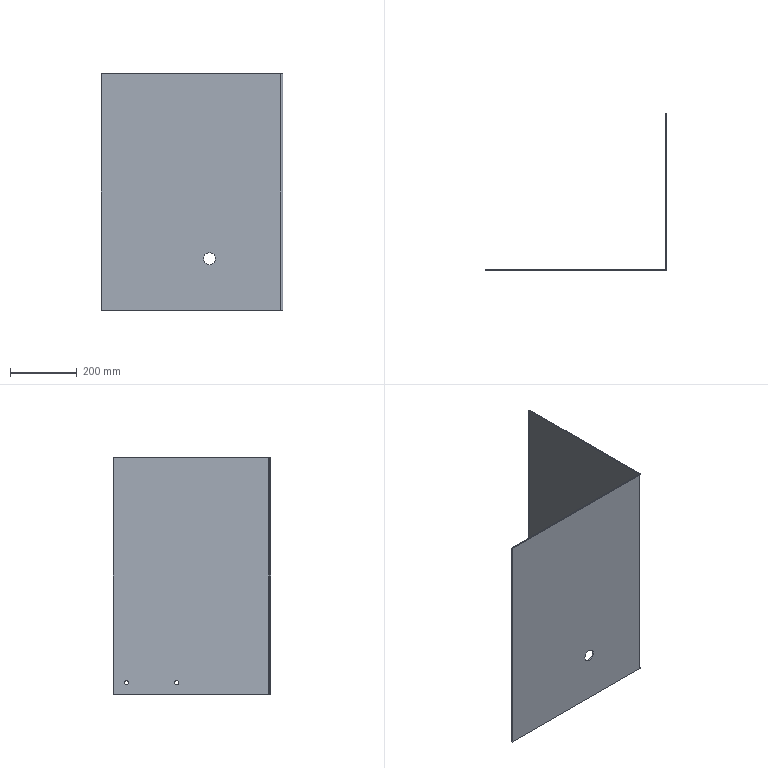Part | SolidWorks | features ICE 2, FlatPattern 1, SMBaseFlange 1, SheetMetal 1 | 1 solid | 20 faces | box 545 x 472 x 710 mm | volume 2151858 mm3 | plane 12 | cylinder 8 | commonest cylinder face diameters 12.7 x4 36.2 x2 6 x1 12 x1
STEP:
#1=CARTESIAN_POINT('',(-3.,432.,41.35));
#2=VERTEX_POINT('',#1);
#3=CARTESIAN_POINT('',(-3.,432.,28.65));
#4=VERTEX_POINT('',#3);
#5=CARTESIAN_POINT('',(-3.,432.,35.));
#6=DIRECTION('',(1.,0.,0.));
#7=DIRECTION('',(0.,0.,-1.));
#8=AXIS2_PLACEMENT_3D('',#5,#6,#7);
#9=CIRCLE('',#8,6.35);
#10=EDGE_CURVE('',#2,#4,#9,.T.);
#11=ORIENTED_EDGE('',*,*,#10,.F.);
#12=CARTESIAN_POINT('',(0.,432.,41.35));
#13=VERTEX_POINT('',#12);
#14=CARTESIAN_POINT('',(-10.,432.,41.35));
#15=DIRECTION('',(1.,0.,0.));
#16=VECTOR('',#15,1000.);
#17=LINE('',#14,#16);
#18=EDGE_CURVE('',#2,#13,#17,.T.);
#19=ORIENTED_EDGE('',*,*,#18,.T.);
#20=CARTESIAN_POINT('',(0.,432.,28.65));
#21=VERTEX_POINT('',#20);
#22=CARTESIAN_POINT('',(0.,432.,35.));
#23=DIRECTION('',(1.,0.,0.));
#24=DIRECTION('',(0.,0.,1.));
#25=AXIS2_PLACEMENT_3D('',#22,#23,#24);
#26=CIRCLE('',#25,6.35);
#27=EDGE_CURVE('',#13,#21,#26,.T.);
#28=ORIENTED_EDGE('',*,*,#27,.T.);
#29=CARTESIAN_POINT('',(-10.,432.,28.65));
#30=DIRECTION('',(1.,0.,0.));
#31=VECTOR('',#30,1000.);
#32=LINE('',#29,#31);
#33=EDGE_CURVE('',#4,#21,#32,.T.);
#34=ORIENTED_EDGE('',*,*,#33,.F.);
#35=EDGE_LOOP('',(#11,#19,#28,#34));
#36=FACE_OUTER_BOUND('',#35,.T.);
#37=CARTESIAN_POINT('',(-10.,432.,35.));
#38=DIRECTION('',(1.,0.,0.));
#39=DIRECTION('',(0.,0.,-1.));
#40=AXIS2_PLACEMENT_3D('',#37,#38,#39);
#41=CYLINDRICAL_SURFACE('',#40,6.35);
#42=ADVANCED_FACE('',(#36),#41,.F.);
#43=CARTESIAN_POINT('',(-3.,282.,41.35));
#44=VERTEX_POINT('',#43);
#45=CARTESIAN_POINT('',(-3.,282.,28.65));
#46=VERTEX_POINT('',#45);
#47=CARTESIAN_POINT('',(-3.,282.,35.));
#48=DIRECTION('',(1.,0.,0.));
#49=DIRECTION('',(0.,0.,-1.));
#50=AXIS2_PLACEMENT_3D('',#47,#48,#49);
#51=CIRCLE('',#50,6.35);
#52=EDGE_CURVE('',#44,#46,#51,.T.);
#53=ORIENTED_EDGE('',*,*,#52,.F.);
#54=CARTESIAN_POINT('',(0.,282.,41.35));
#55=VERTEX_POINT('',#54);
#56=CARTESIAN_POINT('',(-10.,282.,41.35));
#57=DIRECTION('',(1.,0.,0.));
#58=VECTOR('',#57,1000.);
#59=LINE('',#56,#58);
#60=EDGE_CURVE('',#44,#55,#59,.T.);
#61=ORIENTED_EDGE('',*,*,#60,.T.);
#62=CARTESIAN_POINT('',(0.,282.,28.65));
#63=VERTEX_POINT('',#62);
#64=CARTESIAN_POINT('',(0.,282.,35.));
#65=DIRECTION('',(1.,0.,0.));
#66=DIRECTION('',(0.,0.,1.));
#67=AXIS2_PLACEMENT_3D('',#64,#65,#66);
#68=CIRCLE('',#67,6.35);
#69=EDGE_CURVE('',#55,#63,#68,.T.);
#70=ORIENTED_EDGE('',*,*,#69,.T.);
#71=CARTESIAN_POINT('',(-10.,282.,28.65));
#72=DIRECTION('',(1.,0.,0.));
#73=VECTOR('',#72,1000.);
#74=LINE('',#71,#73);
#75=EDGE_CURVE('',#46,#63,#74,.T.);
#76=ORIENTED_EDGE('',*,*,#75,.F.);
#77=EDGE_LOOP('',(#53,#61,#70,#76));
#78=FACE_OUTER_BOUND('',#77,.T.);
#79=CARTESIAN_POINT('',(-10.,282.,35.));
#80=DIRECTION('',(1.,0.,0.));
#81=DIRECTION('',(0.,0.,-1.));
#82=AXIS2_PLACEMENT_3D('',#79,#80,#81);
#83=CYLINDRICAL_SURFACE('',#82,6.35);
#84=ADVANCED_FACE('',(#78),#83,.F.);
#85=CARTESIAN_POINT('',(-238.1,3.,155.));
#86=VERTEX_POINT('',#85);
#87=CARTESIAN_POINT('',(-201.9,3.,155.));
#88=VERTEX_POINT('',#87);
#89=CARTESIAN_POINT('',(-220.,3.,155.));
#90=DIRECTION('',(0.,-1.,0.));
#91=DIRECTION('',(1.,0.,0.));
#92=AXIS2_PLACEMENT_3D('',#89,#90,#91);
#93=CIRCLE('',#92,18.1);
#94=EDGE_CURVE('',#86,#88,#93,.T.);
#95=ORIENTED_EDGE('',*,*,#94,.F.);
#96=CARTESIAN_POINT('',(-238.1,0.,155.));
#97=VERTEX_POINT('',#96);
#98=CARTESIAN_POINT('',(-238.1,10.,155.));
#99=DIRECTION('',(0.,-1.,0.));
#100=VECTOR('',#99,1000.);
#101=LINE('',#98,#100);
#102=EDGE_CURVE('',#86,#97,#101,.T.);
#103=ORIENTED_EDGE('',*,*,#102,.T.);
#104=CARTESIAN_POINT('',(-201.9,0.,155.));
#105=VERTEX_POINT('',#104);
#106=CARTESIAN_POINT('',(-220.,0.,155.));
#107=DIRECTION('',(0.,-1.,0.));
#108=DIRECTION('',(-1.,0.,0.));
#109=AXIS2_PLACEMENT_3D('',#106,#107,#108);
#110=CIRCLE('',#109,18.1);
#111=EDGE_CURVE('',#97,#105,#110,.T.);
#112=ORIENTED_EDGE('',*,*,#111,.T.);
#113=CARTESIAN_POINT('',(-201.9,10.,155.));
#114=DIRECTION('',(0.,-1.,0.));
#115=VECTOR('',#114,1000.);
#116=LINE('',#113,#115);
#117=EDGE_CURVE('',#88,#105,#116,.T.);
#118=ORIENTED_EDGE('',*,*,#117,.F.);
#119=EDGE_LOOP('',(#95,#103,#112,#118));
#120=FACE_OUTER_BOUND('',#119,.T.);
#121=CARTESIAN_POINT('',(-220.,10.,155.));
#122=DIRECTION('',(0.,-1.,0.));
#123=DIRECTION('',(1.,0.,0.));
#124=AXIS2_PLACEMENT_3D('',#121,#122,#123);
#125=CYLINDRICAL_SURFACE('',#124,18.1);
#126=ADVANCED_FACE('',(#120),#125,.F.);
#127=CARTESIAN_POINT('',(-6.,0.,710.));
#128=VERTEX_POINT('',#127);
#129=CARTESIAN_POINT('',(-6.,3.,710.));
#130=VERTEX_POINT('',#129);
#131=CARTESIAN_POINT('',(-6.,0.,710.));
#132=DIRECTION('',(0.,1.,0.));
#133=VECTOR('',#132,1000.);
#134=LINE('',#131,#133);
#135=EDGE_CURVE('',#128,#130,#134,.T.);
#136=ORIENTED_EDGE('',*,*,#135,.F.);
#137=CARTESIAN_POINT('',(0.,6.,710.));
#138=VERTEX_POINT('',#137);
#139=CARTESIAN_POINT('',(-6.,6.,710.));
#140=DIRECTION('',(0.,0.,-1.));
#141=DIRECTION('',(1.,0.,0.));
#142=AXIS2_PLACEMENT_3D('',#139,#140,#141);
#143=CIRCLE('',#142,6.);
#144=EDGE_CURVE('',#138,#128,#143,.T.);
#145=ORIENTED_EDGE('',*,*,#144,.F.);
#146=CARTESIAN_POINT('',(-3.,6.,710.));
#147=VERTEX_POINT('',#146);
#148=CARTESIAN_POINT('',(-3.,6.,710.));
#149=DIRECTION('',(1.,0.,0.));
#150=VECTOR('',#149,1000.);
#151=LINE('',#148,#150);
#152=EDGE_CURVE('',#147,#138,#151,.T.);
#153=ORIENTED_EDGE('',*,*,#152,.F.);
#154=CARTESIAN_POINT('',(-6.,6.,710.));
#155=DIRECTION('',(0.,0.,-1.));
#156=DIRECTION('',(1.,0.,0.));
#157=AXIS2_PLACEMENT_3D('',#154,#155,#156);
#158=CIRCLE('',#157,3.);
#159=EDGE_CURVE('',#147,#130,#158,.T.);
#160=ORIENTED_EDGE('',*,*,#159,.T.);
#161=EDGE_LOOP('',(#136,#145,#153,#160));
#162=FACE_OUTER_BOUND('',#161,.T.);
#163=CARTESIAN_POINT('',(-6.,0.,710.));
#164=DIRECTION('',(0.,0.,1.));
#165=DIRECTION('',(1.,0.,0.));
#166=AXIS2_PLACEMENT_3D('',#163,#164,#165);
#167=PLANE('',#166);
#168=ADVANCED_FACE('',(#162),#167,.T.);
#169=CARTESIAN_POINT('',(-545.,0.,710.));
#170=VERTEX_POINT('',#169);
#171=CARTESIAN_POINT('',(0.,0.,710.));
#172=DIRECTION('',(-1.,0.,0.));
#173=VECTOR('',#172,1000.);
#174=LINE('',#171,#173);
#175=EDGE_CURVE('',#128,#170,#174,.T.);
#176=ORIENTED_EDGE('',*,*,#175,.F.);
#177=ORIENTED_EDGE('',*,*,#135,.T.);
#178=CARTESIAN_POINT('',(-545.,3.,710.));
#179=VERTEX_POINT('',#178);
#180=CARTESIAN_POINT('',(0.,3.,710.));
#181=DIRECTION('',(-1.,0.,0.));
#182=VECTOR('',#181,1000.);
#183=LINE('',#180,#182);
#184=EDGE_CURVE('',#130,#179,#183,.T.);
#185=ORIENTED_EDGE('',*,*,#184,.T.);
#186=CARTESIAN_POINT('',(-545.,0.,710.));
#187=DIRECTION('',(0.,1.,0.));
#188=VECTOR('',#187,1000.);
#189=LINE('',#186,#188);
#190=EDGE_CURVE('',#170,#179,#189,.T.);
#191=ORIENTED_EDGE('',*,*,#190,.F.);
#192=EDGE_LOOP('',(#176,#177,#185,#191));
#193=FACE_OUTER_BOUND('',#192,.T.);
#194=CARTESIAN_POINT('',(-3.,6.,710.));
#195=DIRECTION('',(0.,0.,1.));
#196=DIRECTION('',(1.,0.,0.));
#197=AXIS2_PLACEMENT_3D('',#194,#195,#196);
#198=PLANE('',#197);
#199=ADVANCED_FACE('',(#193),#198,.T.);
#200=CARTESIAN_POINT('',(0.,6.,0.));
#201=VERTEX_POINT('',#200);
#202=CARTESIAN_POINT('',(-3.,6.,0.));
#203=VERTEX_POINT('',#202);
#204=CARTESIAN_POINT('',(0.,6.,0.));
#205=DIRECTION('',(-1.,0.,0.));
#206=VECTOR('',#205,1000.);
#207=LINE('',#204,#206);
#208=EDGE_CURVE('',#201,#203,#207,.T.);
#209=ORIENTED_EDGE('',*,*,#208,.F.);
#210=CARTESIAN_POINT('',(-6.,0.,0.));
#211=VERTEX_POINT('',#210);
#212=CARTESIAN_POINT('',(-6.,6.,0.));
#213=DIRECTION('',(0.,0.,-1.));
#214=DIRECTION('',(1.,0.,0.));
#215=AXIS2_PLACEMENT_3D('',#212,#213,#214);
#216=CIRCLE('',#215,6.);
#217=EDGE_CURVE('',#201,#211,#216,.T.);
#218=ORIENTED_EDGE('',*,*,#217,.T.);
#219=CARTESIAN_POINT('',(-6.,3.,0.));
#220=VERTEX_POINT('',#219);
#221=CARTESIAN_POINT('',(-6.,3.,0.));
#222=DIRECTION('',(0.,-1.,0.));
#223=VECTOR('',#222,1000.);
#224=LINE('',#221,#223);
#225=EDGE_CURVE('',#220,#211,#224,.T.);
#226=ORIENTED_EDGE('',*,*,#225,.F.);
#227=CARTESIAN_POINT('',(-6.,6.,0.));
#228=DIRECTION('',(0.,0.,-1.));
#229=DIRECTION('',(1.,0.,0.));
#230=AXIS2_PLACEMENT_3D('',#227,#228,#229);
#231=CIRCLE('',#230,3.);
#232=EDGE_CURVE('',#203,#220,#231,.T.);
#233=ORIENTED_EDGE('',*,*,#232,.F.);
#234=EDGE_LOOP('',(#209,#218,#226,#233));
#235=FACE_OUTER_BOUND('',#234,.T.);
#236=CARTESIAN_POINT('',(0.,6.,0.));
#237=DIRECTION('',(0.,0.,-1.));
#238=DIRECTION('',(-1.,0.,0.));
#239=AXIS2_PLACEMENT_3D('',#236,#237,#238);
#240=PLANE('',#239);
#241=ADVANCED_FACE('',(#235),#240,.T.);
#242=CARTESIAN_POINT('',(0.,472.,0.));
#243=VERTEX_POINT('',#242);
#244=CARTESIAN_POINT('',(0.,0.,0.));
#245=DIRECTION('',(0.,-1.,0.));
#246=VECTOR('',#245,1000.);
#247=LINE('',#244,#246);
#248=EDGE_CURVE('',#243,#201,#247,.T.);
#249=ORIENTED_EDGE('',*,*,#248,.T.);
#250=ORIENTED_EDGE('',*,*,#208,.T.);
#251=CARTESIAN_POINT('',(-3.,472.,0.));
#252=VERTEX_POINT('',#251);
#253=CARTESIAN_POINT('',(-3.,0.,0.));
#254=DIRECTION('',(0.,-1.,0.));
#255=VECTOR('',#254,1000.);
#256=LINE('',#253,#255);
#257=EDGE_CURVE('',#252,#203,#256,.T.);
#258=ORIENTED_EDGE('',*,*,#257,.F.);
#259=CARTESIAN_POINT('',(-3.,472.,0.));
#260=DIRECTION('',(1.,0.,0.));
#261=VECTOR('',#260,1000.);
#262=LINE('',#259,#261);
#263=EDGE_CURVE('',#252,#243,#262,.T.);
#264=ORIENTED_EDGE('',*,*,#263,.T.);
#265=EDGE_LOOP('',(#249,#250,#258,#264));
#266=FACE_OUTER_BOUND('',#265,.T.);
#267=CARTESIAN_POINT('',(-6.,3.,0.));
#268=DIRECTION('',(0.,0.,-1.));
#269=DIRECTION('',(-1.,0.,0.));
#270=AXIS2_PLACEMENT_3D('',#267,#268,#269);
#271=PLANE('',#270);
#272=ADVANCED_FACE('',(#266),#271,.T.);
#273=CARTESIAN_POINT('',(-220.,3.,155.));
#274=DIRECTION('',(0.,-1.,0.));
#275=DIRECTION('',(1.,0.,0.));
#276=AXIS2_PLACEMENT_3D('',#273,#274,#275);
#277=CIRCLE('',#276,18.1);
#278=EDGE_CURVE('',#88,#86,#277,.T.);
#279=ORIENTED_EDGE('',*,*,#278,.T.);
#280=ORIENTED_EDGE('',*,*,#94,.T.);
#281=EDGE_LOOP('',(#279,#280));
#282=FACE_BOUND('',#281,.T.);
#283=CARTESIAN_POINT('',(-545.,3.,0.));
#284=VERTEX_POINT('',#283);
#285=CARTESIAN_POINT('',(0.,3.,0.));
#286=DIRECTION('',(-1.,0.,0.));
#287=VECTOR('',#286,1000.);
#288=LINE('',#285,#287);
#289=EDGE_CURVE('',#220,#284,#288,.T.);
#290=ORIENTED_EDGE('',*,*,#289,.T.);
#291=CARTESIAN_POINT('',(-545.,3.,710.));
#292=DIRECTION('',(0.,0.,-1.));
#293=VECTOR('',#292,1000.);
#294=LINE('',#291,#293);
#295=EDGE_CURVE('',#179,#284,#294,.T.);
#296=ORIENTED_EDGE('',*,*,#295,.F.);
#297=ORIENTED_EDGE('',*,*,#184,.F.);
#298=CARTESIAN_POINT('',(-6.,3.,710.));
#299=DIRECTION('',(0.,0.,-1.));
#300=VECTOR('',#299,1000.);
#301=LINE('',#298,#300);
#302=EDGE_CURVE('',#130,#220,#301,.T.);
#303=ORIENTED_EDGE('',*,*,#302,.T.);
#304=EDGE_LOOP('',(#290,#296,#297,#303));
#305=FACE_OUTER_BOUND('',#304,.T.);
#306=CARTESIAN_POINT('',(0.,3.,710.));
#307=DIRECTION('',(0.,-1.,0.));
#308=DIRECTION('',(1.,0.,0.));
#309=AXIS2_PLACEMENT_3D('',#306,#307,#308);
#310=PLANE('',#309);
#311=ADVANCED_FACE('',(#282,#305),#310,.F.);
#312=CARTESIAN_POINT('',(-545.,0.,0.));
#313=VERTEX_POINT('',#312);
#314=CARTESIAN_POINT('',(-545.,0.,0.));
#315=DIRECTION('',(0.,1.,0.));
#316=VECTOR('',#315,1000.);
#317=LINE('',#314,#316);
#318=EDGE_CURVE('',#313,#284,#317,.T.);
#319=ORIENTED_EDGE('',*,*,#318,.F.);
#320=CARTESIAN_POINT('',(-545.,0.,710.));
#321=DIRECTION('',(0.,0.,-1.));
#322=VECTOR('',#321,1000.);
#323=LINE('',#320,#322);
#324=EDGE_CURVE('',#170,#313,#323,.T.);
#325=ORIENTED_EDGE('',*,*,#324,.F.);
#326=ORIENTED_EDGE('',*,*,#190,.T.);
#327=ORIENTED_EDGE('',*,*,#295,.T.);
#328=EDGE_LOOP('',(#319,#325,#326,#327));
#329=FACE_OUTER_BOUND('',#328,.T.);
#330=CARTESIAN_POINT('',(-545.,0.,710.));
#331=DIRECTION('',(-1.,0.,0.));
#332=DIRECTION('',(0.,0.,1.));
#333=AXIS2_PLACEMENT_3D('',#330,#331,#332);
#334=PLANE('',#333);
#335=ADVANCED_FACE('',(#329),#334,.T.);
#336=CARTESIAN_POINT('',(-220.,0.,155.));
#337=DIRECTION('',(0.,-1.,0.));
#338=DIRECTION('',(-1.,0.,0.));
#339=AXIS2_PLACEMENT_3D('',#336,#337,#338);
#340=CIRCLE('',#339,18.1);
#341=EDGE_CURVE('',#105,#97,#340,.T.);
#342=ORIENTED_EDGE('',*,*,#341,.F.);
#343=ORIENTED_EDGE('',*,*,#111,.F.);
#344=EDGE_LOOP('',(#342,#343));
#345=FACE_BOUND('',#344,.T.);
#346=CARTESIAN_POINT('',(0.,0.,0.));
#347=DIRECTION('',(-1.,0.,0.));
#348=VECTOR('',#347,1000.);
#349=LINE('',#346,#348);
#350=EDGE_CURVE('',#211,#313,#349,.T.);
#351=ORIENTED_EDGE('',*,*,#350,.F.);
#352=CARTESIAN_POINT('',(-6.,0.,710.));
#353=DIRECTION('',(0.,0.,-1.));
#354=VECTOR('',#353,1000.);
#355=LINE('',#352,#354);
#356=EDGE_CURVE('',#128,#211,#355,.T.);
#357=ORIENTED_EDGE('',*,*,#356,.F.);
#358=ORIENTED_EDGE('',*,*,#175,.T.);
#359=ORIENTED_EDGE('',*,*,#324,.T.);
#360=EDGE_LOOP('',(#351,#357,#358,#359));
#361=FACE_OUTER_BOUND('',#360,.T.);
#362=CARTESIAN_POINT('',(0.,0.,710.));
#363=DIRECTION('',(0.,-1.,0.));
#364=DIRECTION('',(1.,0.,0.));
#365=AXIS2_PLACEMENT_3D('',#362,#363,#364);
#366=PLANE('',#365);
#367=ADVANCED_FACE('',(#345,#361),#366,.T.);
#368=ORIENTED_EDGE('',*,*,#217,.F.);
#369=CARTESIAN_POINT('',(0.,6.,710.));
#370=DIRECTION('',(0.,0.,-1.));
#371=VECTOR('',#370,1000.);
#372=LINE('',#369,#371);
#373=EDGE_CURVE('',#138,#201,#372,.T.);
#374=ORIENTED_EDGE('',*,*,#373,.F.);
#375=ORIENTED_EDGE('',*,*,#144,.T.);
#376=ORIENTED_EDGE('',*,*,#356,.T.);
#377=EDGE_LOOP('',(#368,#374,#375,#376));
#378=FACE_OUTER_BOUND('',#377,.T.);
#379=CARTESIAN_POINT('',(-6.,6.,710.));
#380=DIRECTION('',(0.,0.,-1.));
#381=DIRECTION('',(-1.,0.,0.));
#382=AXIS2_PLACEMENT_3D('',#379,#380,#381);
#383=CYLINDRICAL_SURFACE('',#382,6.);
#384=ADVANCED_FACE('',(#378),#383,.T.);
#385=CARTESIAN_POINT('',(0.,432.,35.));
#386=DIRECTION('',(1.,0.,0.));
#387=DIRECTION('',(0.,0.,1.));
#388=AXIS2_PLACEMENT_3D('',#385,#386,#387);
#389=CIRCLE('',#388,6.35);
#390=EDGE_CURVE('',#21,#13,#389,.T.);
#391=ORIENTED_EDGE('',*,*,#390,.F.);
#392=ORIENTED_EDGE('',*,*,#27,.F.);
#393=EDGE_LOOP('',(#391,#392));
#394=FACE_BOUND('',#393,.T.);
#395=CARTESIAN_POINT('',(0.,282.,35.));
#396=DIRECTION('',(1.,0.,0.));
#397=DIRECTION('',(0.,0.,1.));
#398=AXIS2_PLACEMENT_3D('',#395,#396,#397);
#399=CIRCLE('',#398,6.35);
#400=EDGE_CURVE('',#63,#55,#399,.T.);
#401=ORIENTED_EDGE('',*,*,#400,.F.);
#402=ORIENTED_EDGE('',*,*,#69,.F.);
#403=EDGE_LOOP('',(#401,#402));
#404=FACE_BOUND('',#403,.T.);
#405=ORIENTED_EDGE('',*,*,#248,.F.);
#406=CARTESIAN_POINT('',(0.,472.,710.));
#407=VERTEX_POINT('',#406);
#408=CARTESIAN_POINT('',(0.,472.,710.));
#409=DIRECTION('',(0.,0.,-1.));
#410=VECTOR('',#409,1000.);
#411=LINE('',#408,#410);
#412=EDGE_CURVE('',#407,#243,#411,.T.);
#413=ORIENTED_EDGE('',*,*,#412,.F.);
#414=CARTESIAN_POINT('',(0.,0.,710.));
#415=DIRECTION('',(0.,-1.,0.));
#416=VECTOR('',#415,1000.);
#417=LINE('',#414,#416);
#418=EDGE_CURVE('',#407,#138,#417,.T.);
#419=ORIENTED_EDGE('',*,*,#418,.T.);
#420=ORIENTED_EDGE('',*,*,#373,.T.);
#421=EDGE_LOOP('',(#405,#413,#419,#420));
#422=FACE_OUTER_BOUND('',#421,.T.);
#423=CARTESIAN_POINT('',(0.,0.,710.));
#424=DIRECTION('',(1.,0.,0.));
#425=DIRECTION('',(0.,0.,-1.));
#426=AXIS2_PLACEMENT_3D('',#423,#424,#425);
#427=PLANE('',#426);
#428=ADVANCED_FACE('',(#394,#404,#422),#427,.T.);
#429=ORIENTED_EDGE('',*,*,#263,.F.);
#430=CARTESIAN_POINT('',(-3.,472.,710.));
#431=VERTEX_POINT('',#430);
#432=CARTESIAN_POINT('',(-3.,472.,710.));
#433=DIRECTION('',(0.,0.,-1.));
#434=VECTOR('',#433,1000.);
#435=LINE('',#432,#434);
#436=EDGE_CURVE('',#431,#252,#435,.T.);
#437=ORIENTED_EDGE('',*,*,#436,.F.);
#438=CARTESIAN_POINT('',(-3.,472.,710.));
#439=DIRECTION('',(1.,0.,0.));
#440=VECTOR('',#439,1000.);
#441=LINE('',#438,#440);
#442=EDGE_CURVE('',#431,#407,#441,.T.);
#443=ORIENTED_EDGE('',*,*,#442,.T.);
#444=ORIENTED_EDGE('',*,*,#412,.T.);
#445=EDGE_LOOP('',(#429,#437,#443,#444));
#446=FACE_OUTER_BOUND('',#445,.T.);
#447=CARTESIAN_POINT('',(-3.,472.,710.));
#448=DIRECTION('',(0.,1.,0.));
#449=DIRECTION('',(0.,0.,1.));
#450=AXIS2_PLACEMENT_3D('',#447,#448,#449);
#451=PLANE('',#450);
#452=ADVANCED_FACE('',(#446),#451,.T.);
#453=CARTESIAN_POINT('',(-3.,432.,35.));
#454=DIRECTION('',(1.,0.,0.));
#455=DIRECTION('',(0.,0.,-1.));
#456=AXIS2_PLACEMENT_3D('',#453,#454,#455);
#457=CIRCLE('',#456,6.35);
#458=EDGE_CURVE('',#4,#2,#457,.T.);
#459=ORIENTED_EDGE('',*,*,#458,.T.);
#460=ORIENTED_EDGE('',*,*,#10,.T.);
#461=EDGE_LOOP('',(#459,#460));
#462=FACE_BOUND('',#461,.T.);
#463=CARTESIAN_POINT('',(-3.,282.,35.));
#464=DIRECTION('',(1.,0.,0.));
#465=DIRECTION('',(0.,0.,-1.));
#466=AXIS2_PLACEMENT_3D('',#463,#464,#465);
#467=CIRCLE('',#466,6.35);
#468=EDGE_CURVE('',#46,#44,#467,.T.);
#469=ORIENTED_EDGE('',*,*,#468,.T.);
#470=ORIENTED_EDGE('',*,*,#52,.T.);
#471=EDGE_LOOP('',(#469,#470));
#472=FACE_BOUND('',#471,.T.);
#473=ORIENTED_EDGE('',*,*,#257,.T.);
#474=CARTESIAN_POINT('',(-3.,6.,710.));
#475=DIRECTION('',(0.,0.,-1.));
#476=VECTOR('',#475,1000.);
#477=LINE('',#474,#476);
#478=EDGE_CURVE('',#147,#203,#477,.T.);
#479=ORIENTED_EDGE('',*,*,#478,.F.);
#480=CARTESIAN_POINT('',(-3.,0.,710.));
#481=DIRECTION('',(0.,-1.,0.));
#482=VECTOR('',#481,1000.);
#483=LINE('',#480,#482);
#484=EDGE_CURVE('',#431,#147,#483,.T.);
#485=ORIENTED_EDGE('',*,*,#484,.F.);
#486=ORIENTED_EDGE('',*,*,#436,.T.);
#487=EDGE_LOOP('',(#473,#479,#485,#486));
#488=FACE_OUTER_BOUND('',#487,.T.);
#489=CARTESIAN_POINT('',(-3.,0.,710.));
#490=DIRECTION('',(1.,0.,0.));
#491=DIRECTION('',(0.,0.,-1.));
#492=AXIS2_PLACEMENT_3D('',#489,#490,#491);
#493=PLANE('',#492);
#494=ADVANCED_FACE('',(#462,#472,#488),#493,.F.);
#495=ORIENTED_EDGE('',*,*,#232,.T.);
#496=ORIENTED_EDGE('',*,*,#302,.F.);
#497=ORIENTED_EDGE('',*,*,#159,.F.);
#498=ORIENTED_EDGE('',*,*,#478,.T.);
#499=EDGE_LOOP('',(#495,#496,#497,#498));
#500=FACE_OUTER_BOUND('',#499,.T.);
#501=CARTESIAN_POINT('',(-6.,6.,710.));
#502=DIRECTION('',(0.,0.,-1.));
#503=DIRECTION('',(-1.,0.,0.));
#504=AXIS2_PLACEMENT_3D('',#501,#502,#503);
#505=CYLINDRICAL_SURFACE('',#504,3.);
#506=ADVANCED_FACE('',(#500),#505,.F.);
#507=ORIENTED_EDGE('',*,*,#484,.T.);
#508=ORIENTED_EDGE('',*,*,#152,.T.);
#509=ORIENTED_EDGE('',*,*,#418,.F.);
#510=ORIENTED_EDGE('',*,*,#442,.F.);
#511=EDGE_LOOP('',(#507,#508,#509,#510));
#512=FACE_OUTER_BOUND('',#511,.T.);
#513=CARTESIAN_POINT('',(-6.,6.,710.));
#514=DIRECTION('',(0.,0.,1.));
#515=DIRECTION('',(1.,0.,0.));
#516=AXIS2_PLACEMENT_3D('',#513,#514,#515);
#517=PLANE('',#516);
#518=ADVANCED_FACE('',(#512),#517,.T.);
#519=ORIENTED_EDGE('',*,*,#289,.F.);
#520=ORIENTED_EDGE('',*,*,#225,.T.);
#521=ORIENTED_EDGE('',*,*,#350,.T.);
#522=ORIENTED_EDGE('',*,*,#318,.T.);
#523=EDGE_LOOP('',(#519,#520,#521,#522));
#524=FACE_OUTER_BOUND('',#523,.T.);
#525=CARTESIAN_POINT('',(-6.,6.,0.));
#526=DIRECTION('',(0.,0.,1.));
#527=DIRECTION('',(1.,0.,0.));
#528=AXIS2_PLACEMENT_3D('',#525,#526,#527);
#529=PLANE('',#528);
#530=ADVANCED_FACE('',(#524),#529,.F.);
#531=ORIENTED_EDGE('',*,*,#102,.F.);
#532=ORIENTED_EDGE('',*,*,#278,.F.);
#533=ORIENTED_EDGE('',*,*,#117,.T.);
#534=ORIENTED_EDGE('',*,*,#341,.T.);
#535=EDGE_LOOP('',(#531,#532,#533,#534));
#536=FACE_OUTER_BOUND('',#535,.T.);
#537=CARTESIAN_POINT('',(-220.,10.,155.));
#538=DIRECTION('',(0.,-1.,0.));
#539=DIRECTION('',(1.,0.,0.));
#540=AXIS2_PLACEMENT_3D('',#537,#538,#539);
#541=CYLINDRICAL_SURFACE('',#540,18.1);
#542=ADVANCED_FACE('',(#536),#541,.F.);
#543=ORIENTED_EDGE('',*,*,#60,.F.);
#544=ORIENTED_EDGE('',*,*,#468,.F.);
#545=ORIENTED_EDGE('',*,*,#75,.T.);
#546=ORIENTED_EDGE('',*,*,#400,.T.);
#547=EDGE_LOOP('',(#543,#544,#545,#546));
#548=FACE_OUTER_BOUND('',#547,.T.);
#549=CARTESIAN_POINT('',(-10.,282.,35.));
#550=DIRECTION('',(1.,0.,0.));
#551=DIRECTION('',(0.,0.,-1.));
#552=AXIS2_PLACEMENT_3D('',#549,#550,#551);
#553=CYLINDRICAL_SURFACE('',#552,6.35);
#554=ADVANCED_FACE('',(#548),#553,.F.);
#555=ORIENTED_EDGE('',*,*,#18,.F.);
#556=ORIENTED_EDGE('',*,*,#458,.F.);
#557=ORIENTED_EDGE('',*,*,#33,.T.);
#558=ORIENTED_EDGE('',*,*,#390,.T.);
#559=EDGE_LOOP('',(#555,#556,#557,#558));
#560=FACE_OUTER_BOUND('',#559,.T.);
#561=CARTESIAN_POINT('',(-10.,432.,35.));
#562=DIRECTION('',(1.,0.,0.));
#563=DIRECTION('',(0.,0.,-1.));
#564=AXIS2_PLACEMENT_3D('',#561,#562,#563);
#565=CYLINDRICAL_SURFACE('',#564,6.35);
#566=ADVANCED_FACE('',(#560),#565,.F.);
#567=CLOSED_SHELL('',(#42,#84,#126,#168,#199,#241,#272,#311,#335,#367,#384,#428,#452,#494,#506,#518,#530,#542,#554,#566));
#568=MANIFOLD_SOLID_BREP('',#567);
#569=CARTESIAN_POINT('',(0.,0.,0.));
#570=DIRECTION('',(0.,0.,1.));
#571=DIRECTION('',(1.,0.,0.));
#572=AXIS2_PLACEMENT_3D('',#569,#570,#571);
#573=(LENGTH_UNIT()NAMED_UNIT(*)SI_UNIT(.MILLI.,.METRE.));
#574=UNCERTAINTY_MEASURE_WITH_UNIT(LENGTH_MEASURE(0.00001),#573,'','');
#575=(NAMED_UNIT(*)PLANE_ANGLE_UNIT()SI_UNIT($,.RADIAN.));
#576=(NAMED_UNIT(*)SI_UNIT($,.STERADIAN.)SOLID_ANGLE_UNIT());
#577=(GEOMETRIC_REPRESENTATION_CONTEXT(3)GLOBAL_UNCERTAINTY_ASSIGNED_CONTEXT((#574))GLOBAL_UNIT_ASSIGNED_CONTEXT((#573,#575,#576))REPRESENTATION_CONTEXT('',''));
#578=ADVANCED_BREP_SHAPE_REPRESENTATION('',(#568,#572),#577);